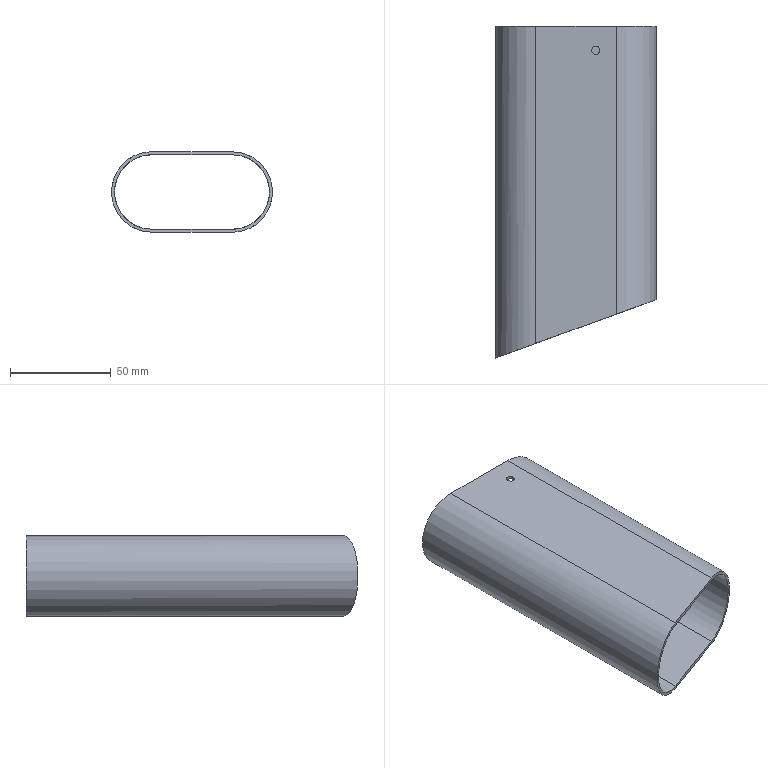Part | STEP file | 6100104L | 1 solid | 11 faces | box 80 x 165 x 40 mm | volume 45327 mm3 | plane 6 | cylinder 5 | commonest cylinder face diameters 37 x2 40 x2 4 x1
STEP:
#1=CARTESIAN_POINT('',(0.,0.,0.));
#2=DIRECTION('',(0.,0.,1.));
#3=DIRECTION('',(1.,0.,0.));
#4=AXIS2_PLACEMENT_3D('',#1,#2,#3);
#5=CARTESIAN_POINT('',(-20.,165.,-20.));
#6=VERTEX_POINT('',#5);
#7=CARTESIAN_POINT('',(-20.,165.,20.));
#8=VERTEX_POINT('',#7);
#9=CARTESIAN_POINT('',(-20.,165.,0.));
#10=DIRECTION('',(0.,1.,0.));
#11=DIRECTION('',(0.,0.,1.));
#12=AXIS2_PLACEMENT_3D('',#9,#10,#11);
#13=CIRCLE('',#12,20.);
#14=CARTESIAN_POINT('',(-20.,165.,0.));
#15=DIRECTION('',(0.,1.,0.));
#16=DIRECTION('',(0.,0.,1.));
#17=AXIS2_PLACEMENT_3D('',#14,#15,#16);
#18=PLANE('',#17);
#19=CARTESIAN_POINT('',(0.,0.));
#20=DIRECTION('',(1.,0.));
#21=AXIS2_PLACEMENT_2D('',#19,#20);
#22=CIRCLE('',#21,20.);
#23=(GEOMETRIC_REPRESENTATION_CONTEXT(2)PARAMETRIC_REPRESENTATION_CONTEXT()REPRESENTATION_CONTEXT('',''));
#24=DEFINITIONAL_REPRESENTATION('',(#22),#23);
#25=PCURVE('',#18,#24);
#26=CARTESIAN_POINT('',(-20.,165.,0.));
#27=DIRECTION('',(0.,-1.,0.));
#28=DIRECTION('',(0.,0.,-1.));
#29=AXIS2_PLACEMENT_3D('',#26,#27,#28);
#30=CYLINDRICAL_SURFACE('',#29,20.);
#31=CARTESIAN_POINT('',(9.425,0.));
#32=DIRECTION('',(-1.,0.));
#33=VECTOR('',#32,1.);
#34=LINE('',#31,#33);
#35=(GEOMETRIC_REPRESENTATION_CONTEXT(2)PARAMETRIC_REPRESENTATION_CONTEXT()REPRESENTATION_CONTEXT('',''));
#36=DEFINITIONAL_REPRESENTATION('',(#34),#35);
#37=PCURVE('',#30,#36);
#38=SURFACE_CURVE('',#13,(#25,#37),.PCURVE_S1.);
#39=EDGE_CURVE('',#6,#8,#38,.T.);
#40=ORIENTED_EDGE('',*,*,#39,.T.);
#41=CARTESIAN_POINT('',(20.,165.,20.));
#42=VERTEX_POINT('',#41);
#43=CARTESIAN_POINT('',(-20.,165.,20.));
#44=DIRECTION('',(1.,0.,0.));
#45=VECTOR('',#44,1.);
#46=LINE('',#43,#45);
#47=CARTESIAN_POINT('',(20.,0.));
#48=DIRECTION('',(0.,1.));
#49=VECTOR('',#48,1.);
#50=LINE('',#47,#49);
#51=(GEOMETRIC_REPRESENTATION_CONTEXT(2)PARAMETRIC_REPRESENTATION_CONTEXT()REPRESENTATION_CONTEXT('',''));
#52=DEFINITIONAL_REPRESENTATION('',(#50),#51);
#53=PCURVE('',#18,#52);
#54=CARTESIAN_POINT('',(-20.,165.,20.));
#55=DIRECTION('',(0.,0.,-1.));
#56=DIRECTION('',(-1.,0.,0.));
#57=AXIS2_PLACEMENT_3D('',#54,#55,#56);
#58=PLANE('',#57);
#59=CARTESIAN_POINT('',(0.,0.));
#60=DIRECTION('',(-1.,0.));
#61=VECTOR('',#60,1.);
#62=LINE('',#59,#61);
#63=(GEOMETRIC_REPRESENTATION_CONTEXT(2)PARAMETRIC_REPRESENTATION_CONTEXT()REPRESENTATION_CONTEXT('',''));
#64=DEFINITIONAL_REPRESENTATION('',(#62),#63);
#65=PCURVE('',#58,#64);
#66=SURFACE_CURVE('',#46,(#53,#65),.PCURVE_S1.);
#67=EDGE_CURVE('',#8,#42,#66,.T.);
#68=ORIENTED_EDGE('',*,*,#67,.T.);
#69=CARTESIAN_POINT('',(20.,165.,-20.));
#70=VERTEX_POINT('',#69);
#71=CARTESIAN_POINT('',(20.,165.,0.));
#72=DIRECTION('',(0.,1.,0.));
#73=DIRECTION('',(0.,0.,1.));
#74=AXIS2_PLACEMENT_3D('',#71,#72,#73);
#75=CIRCLE('',#74,20.);
#76=CARTESIAN_POINT('',(0.,40.));
#77=DIRECTION('',(1.,0.));
#78=AXIS2_PLACEMENT_2D('',#76,#77);
#79=CIRCLE('',#78,20.);
#80=(GEOMETRIC_REPRESENTATION_CONTEXT(2)PARAMETRIC_REPRESENTATION_CONTEXT()REPRESENTATION_CONTEXT('',''));
#81=DEFINITIONAL_REPRESENTATION('',(#79),#80);
#82=PCURVE('',#18,#81);
#83=CARTESIAN_POINT('',(20.,165.,0.));
#84=DIRECTION('',(0.,-1.,0.));
#85=DIRECTION('',(0.,0.,-1.));
#86=AXIS2_PLACEMENT_3D('',#83,#84,#85);
#87=CYLINDRICAL_SURFACE('',#86,20.);
#88=CARTESIAN_POINT('',(3.142,0.));
#89=DIRECTION('',(-1.,0.));
#90=VECTOR('',#89,1.);
#91=LINE('',#88,#90);
#92=(GEOMETRIC_REPRESENTATION_CONTEXT(2)PARAMETRIC_REPRESENTATION_CONTEXT()REPRESENTATION_CONTEXT('',''));
#93=DEFINITIONAL_REPRESENTATION('',(#91),#92);
#94=PCURVE('',#87,#93);
#95=SURFACE_CURVE('',#75,(#82,#94),.PCURVE_S1.);
#96=EDGE_CURVE('',#42,#70,#95,.T.);
#97=ORIENTED_EDGE('',*,*,#96,.T.);
#98=CARTESIAN_POINT('',(-20.,165.,-20.));
#99=DIRECTION('',(-1.,0.,0.));
#100=VECTOR('',#99,1.);
#101=LINE('',#98,#100);
#102=CARTESIAN_POINT('',(-20.,0.));
#103=DIRECTION('',(0.,-1.));
#104=VECTOR('',#103,1.);
#105=LINE('',#102,#104);
#106=(GEOMETRIC_REPRESENTATION_CONTEXT(2)PARAMETRIC_REPRESENTATION_CONTEXT()REPRESENTATION_CONTEXT('',''));
#107=DEFINITIONAL_REPRESENTATION('',(#105),#106);
#108=PCURVE('',#18,#107);
#109=CARTESIAN_POINT('',(-20.,165.,-20.));
#110=DIRECTION('',(0.,0.,1.));
#111=DIRECTION('',(1.,0.,0.));
#112=AXIS2_PLACEMENT_3D('',#109,#110,#111);
#113=PLANE('',#112);
#114=CARTESIAN_POINT('',(0.,0.));
#115=DIRECTION('',(-1.,0.));
#116=VECTOR('',#115,1.);
#117=LINE('',#114,#116);
#118=(GEOMETRIC_REPRESENTATION_CONTEXT(2)PARAMETRIC_REPRESENTATION_CONTEXT()REPRESENTATION_CONTEXT('',''));
#119=DEFINITIONAL_REPRESENTATION('',(#117),#118);
#120=PCURVE('',#113,#119);
#121=SURFACE_CURVE('',#101,(#108,#120),.PCURVE_S1.);
#122=EDGE_CURVE('',#70,#6,#121,.T.);
#123=ORIENTED_EDGE('',*,*,#122,.T.);
#124=EDGE_LOOP('',(#40,#68,#97,#123));
#125=FACE_BOUND('',#124,.T.);
#126=CARTESIAN_POINT('',(-20.,165.,18.5));
#127=VERTEX_POINT('',#126);
#128=CARTESIAN_POINT('',(20.,165.,18.5));
#129=VERTEX_POINT('',#128);
#130=CARTESIAN_POINT('',(-20.,165.,18.5));
#131=DIRECTION('',(1.,0.,0.));
#132=VECTOR('',#131,1.);
#133=LINE('',#130,#132);
#134=CARTESIAN_POINT('',(18.5,0.));
#135=DIRECTION('',(0.,1.));
#136=VECTOR('',#135,1.);
#137=LINE('',#134,#136);
#138=(GEOMETRIC_REPRESENTATION_CONTEXT(2)PARAMETRIC_REPRESENTATION_CONTEXT()REPRESENTATION_CONTEXT('',''));
#139=DEFINITIONAL_REPRESENTATION('',(#137),#138);
#140=PCURVE('',#18,#139);
#141=CARTESIAN_POINT('',(-20.,165.,18.5));
#142=DIRECTION('',(0.,0.,-1.));
#143=DIRECTION('',(-1.,0.,0.));
#144=AXIS2_PLACEMENT_3D('',#141,#142,#143);
#145=PLANE('',#144);
#146=CARTESIAN_POINT('',(0.,0.));
#147=DIRECTION('',(-1.,0.));
#148=VECTOR('',#147,1.);
#149=LINE('',#146,#148);
#150=(GEOMETRIC_REPRESENTATION_CONTEXT(2)PARAMETRIC_REPRESENTATION_CONTEXT()REPRESENTATION_CONTEXT('',''));
#151=DEFINITIONAL_REPRESENTATION('',(#149),#150);
#152=PCURVE('',#145,#151);
#153=SURFACE_CURVE('',#133,(#140,#152),.PCURVE_S1.);
#154=EDGE_CURVE('',#127,#129,#153,.T.);
#155=ORIENTED_EDGE('',*,*,#154,.F.);
#156=CARTESIAN_POINT('',(-20.,165.,-18.5));
#157=VERTEX_POINT('',#156);
#158=CARTESIAN_POINT('',(-20.,165.,0.));
#159=DIRECTION('',(0.,1.,0.));
#160=DIRECTION('',(0.,0.,1.));
#161=AXIS2_PLACEMENT_3D('',#158,#159,#160);
#162=CIRCLE('',#161,18.5);
#163=CARTESIAN_POINT('',(0.,0.));
#164=DIRECTION('',(1.,0.));
#165=AXIS2_PLACEMENT_2D('',#163,#164);
#166=CIRCLE('',#165,18.5);
#167=(GEOMETRIC_REPRESENTATION_CONTEXT(2)PARAMETRIC_REPRESENTATION_CONTEXT()REPRESENTATION_CONTEXT('',''));
#168=DEFINITIONAL_REPRESENTATION('',(#166),#167);
#169=PCURVE('',#18,#168);
#170=CARTESIAN_POINT('',(-20.,165.,0.));
#171=DIRECTION('',(0.,-1.,0.));
#172=DIRECTION('',(0.,0.,-1.));
#173=AXIS2_PLACEMENT_3D('',#170,#171,#172);
#174=CYLINDRICAL_SURFACE('',#173,18.5);
#175=CARTESIAN_POINT('',(9.425,0.));
#176=DIRECTION('',(-1.,0.));
#177=VECTOR('',#176,1.);
#178=LINE('',#175,#177);
#179=(GEOMETRIC_REPRESENTATION_CONTEXT(2)PARAMETRIC_REPRESENTATION_CONTEXT()REPRESENTATION_CONTEXT('',''));
#180=DEFINITIONAL_REPRESENTATION('',(#178),#179);
#181=PCURVE('',#174,#180);
#182=SURFACE_CURVE('',#162,(#169,#181),.PCURVE_S1.);
#183=EDGE_CURVE('',#157,#127,#182,.T.);
#184=ORIENTED_EDGE('',*,*,#183,.F.);
#185=CARTESIAN_POINT('',(20.,165.,-18.5));
#186=VERTEX_POINT('',#185);
#187=CARTESIAN_POINT('',(-20.,165.,-18.5));
#188=DIRECTION('',(-1.,0.,0.));
#189=VECTOR('',#188,1.);
#190=LINE('',#187,#189);
#191=CARTESIAN_POINT('',(-18.5,0.));
#192=DIRECTION('',(0.,-1.));
#193=VECTOR('',#192,1.);
#194=LINE('',#191,#193);
#195=(GEOMETRIC_REPRESENTATION_CONTEXT(2)PARAMETRIC_REPRESENTATION_CONTEXT()REPRESENTATION_CONTEXT('',''));
#196=DEFINITIONAL_REPRESENTATION('',(#194),#195);
#197=PCURVE('',#18,#196);
#198=CARTESIAN_POINT('',(-20.,165.,-18.5));
#199=DIRECTION('',(0.,0.,1.));
#200=DIRECTION('',(1.,0.,0.));
#201=AXIS2_PLACEMENT_3D('',#198,#199,#200);
#202=PLANE('',#201);
#203=CARTESIAN_POINT('',(0.,0.));
#204=DIRECTION('',(-1.,0.));
#205=VECTOR('',#204,1.);
#206=LINE('',#203,#205);
#207=(GEOMETRIC_REPRESENTATION_CONTEXT(2)PARAMETRIC_REPRESENTATION_CONTEXT()REPRESENTATION_CONTEXT('',''));
#208=DEFINITIONAL_REPRESENTATION('',(#206),#207);
#209=PCURVE('',#202,#208);
#210=SURFACE_CURVE('',#190,(#197,#209),.PCURVE_S1.);
#211=EDGE_CURVE('',#186,#157,#210,.T.);
#212=ORIENTED_EDGE('',*,*,#211,.F.);
#213=CARTESIAN_POINT('',(20.,165.,0.));
#214=DIRECTION('',(0.,1.,0.));
#215=DIRECTION('',(0.,0.,1.));
#216=AXIS2_PLACEMENT_3D('',#213,#214,#215);
#217=CIRCLE('',#216,18.5);
#218=CARTESIAN_POINT('',(0.,40.));
#219=DIRECTION('',(1.,0.));
#220=AXIS2_PLACEMENT_2D('',#218,#219);
#221=CIRCLE('',#220,18.5);
#222=(GEOMETRIC_REPRESENTATION_CONTEXT(2)PARAMETRIC_REPRESENTATION_CONTEXT()REPRESENTATION_CONTEXT('',''));
#223=DEFINITIONAL_REPRESENTATION('',(#221),#222);
#224=PCURVE('',#18,#223);
#225=CARTESIAN_POINT('',(20.,165.,0.));
#226=DIRECTION('',(0.,-1.,0.));
#227=DIRECTION('',(0.,0.,-1.));
#228=AXIS2_PLACEMENT_3D('',#225,#226,#227);
#229=CYLINDRICAL_SURFACE('',#228,18.5);
#230=CARTESIAN_POINT('',(3.142,0.));
#231=DIRECTION('',(-1.,0.));
#232=VECTOR('',#231,1.);
#233=LINE('',#230,#232);
#234=(GEOMETRIC_REPRESENTATION_CONTEXT(2)PARAMETRIC_REPRESENTATION_CONTEXT()REPRESENTATION_CONTEXT('',''));
#235=DEFINITIONAL_REPRESENTATION('',(#233),#234);
#236=PCURVE('',#229,#235);
#237=SURFACE_CURVE('',#217,(#224,#236),.PCURVE_S1.);
#238=EDGE_CURVE('',#129,#186,#237,.T.);
#239=ORIENTED_EDGE('',*,*,#238,.F.);
#240=EDGE_LOOP('',(#155,#184,#212,#239));
#241=FACE_BOUND('',#240,.T.);
#242=ADVANCED_FACE('',(#125,#241),#18,.T.);
#243=CARTESIAN_POINT('',(-20.,7.279,-20.));
#244=VERTEX_POINT('',#243);
#245=CARTESIAN_POINT('',(-20.,165.,-20.));
#246=DIRECTION('',(0.,-1.,0.));
#247=VECTOR('',#246,1.);
#248=LINE('',#245,#247);
#249=CARTESIAN_POINT('',(6.283,0.));
#250=DIRECTION('',(0.,1.));
#251=VECTOR('',#250,1.);
#252=LINE('',#249,#251);
#253=(GEOMETRIC_REPRESENTATION_CONTEXT(2)PARAMETRIC_REPRESENTATION_CONTEXT()REPRESENTATION_CONTEXT('',''));
#254=DEFINITIONAL_REPRESENTATION('',(#252),#253);
#255=PCURVE('',#30,#254);
#256=CARTESIAN_POINT('',(0.,0.));
#257=DIRECTION('',(0.,-1.));
#258=VECTOR('',#257,1.);
#259=LINE('',#256,#258);
#260=(GEOMETRIC_REPRESENTATION_CONTEXT(2)PARAMETRIC_REPRESENTATION_CONTEXT()REPRESENTATION_CONTEXT('',''));
#261=DEFINITIONAL_REPRESENTATION('',(#259),#260);
#262=PCURVE('',#113,#261);
#263=SURFACE_CURVE('',#248,(#255,#262),.PCURVE_S1.);
#264=EDGE_CURVE('',#6,#244,#263,.T.);
#265=ORIENTED_EDGE('',*,*,#264,.T.);
#266=CARTESIAN_POINT('',(-20.,7.279,20.));
#267=VERTEX_POINT('',#266);
#268=CARTESIAN_POINT('',(-20.,7.279,-20.));
#269=CARTESIAN_POINT('',(-60.,-7.279,-20.));
#270=CARTESIAN_POINT('',(-60.,-7.279,20.));
#271=CARTESIAN_POINT('',(-20.,7.279,20.));
#272=(BOUNDED_CURVE()B_SPLINE_CURVE(3,(#268,#269,#270,#271),.UNSPECIFIED.,.F.,.F.)B_SPLINE_CURVE_WITH_KNOTS((4,4),(4.712,7.854),.PIECEWISE_BEZIER_KNOTS.)CURVE()GEOMETRIC_REPRESENTATION_ITEM()RATIONAL_B_SPLINE_CURVE((1.,0.3333,0.3333,1.))REPRESENTATION_ITEM(''));
#273=CARTESIAN_POINT('',(6.283,157.721));
#274=CARTESIAN_POINT('',(6.253,157.941));
#275=CARTESIAN_POINT('',(6.19,158.403));
#276=CARTESIAN_POINT('',(6.085,159.153));
#277=CARTESIAN_POINT('',(5.972,159.957));
#278=CARTESIAN_POINT('',(5.848,160.8));
#279=CARTESIAN_POINT('',(5.713,161.664));
#280=CARTESIAN_POINT('',(5.567,162.516));
#281=CARTESIAN_POINT('',(5.412,163.316));
#282=CARTESIAN_POINT('',(5.246,164.017));
#283=CARTESIAN_POINT('',(5.073,164.567));
#284=CARTESIAN_POINT('',(4.894,164.919));
#285=CARTESIAN_POINT('',(4.712,165.04));
#286=CARTESIAN_POINT('',(4.531,164.919));
#287=CARTESIAN_POINT('',(4.352,164.567));
#288=CARTESIAN_POINT('',(4.179,164.017));
#289=CARTESIAN_POINT('',(4.013,163.316));
#290=CARTESIAN_POINT('',(3.857,162.516));
#291=CARTESIAN_POINT('',(3.712,161.664));
#292=CARTESIAN_POINT('',(3.577,160.8));
#293=CARTESIAN_POINT('',(3.453,159.957));
#294=CARTESIAN_POINT('',(3.339,159.153));
#295=CARTESIAN_POINT('',(3.235,158.403));
#296=CARTESIAN_POINT('',(3.172,157.941));
#297=CARTESIAN_POINT('',(3.142,157.721));
#298=B_SPLINE_CURVE_WITH_KNOTS('',3,(#273,#274,#275,#276,#277,#278,#279,#280,#281,#282,#283,#284,#285,#286,#287,#288,#289,#290,#291,#292,#293,#294,#295,#296,#297),.UNSPECIFIED.,.F.,.F.,(4,1,1,1,1,1,1,1,1,1,1,1,1,1,1,1,1,1,1,1,1,1,4),(4.712,4.855,4.998,5.141,5.284,5.426,5.569,5.712,5.855,5.998,6.14,6.283,6.426,6.569,6.712,6.854,6.997,7.14,7.283,7.426,7.568,7.711,7.854),.QUASI_UNIFORM_KNOTS.);
#299=(GEOMETRIC_REPRESENTATION_CONTEXT(2)PARAMETRIC_REPRESENTATION_CONTEXT()REPRESENTATION_CONTEXT('',''));
#300=DEFINITIONAL_REPRESENTATION('',(#298),#299);
#301=PCURVE('',#30,#300);
#302=CARTESIAN_POINT('',(-40.,0.,-40.));
#303=DIRECTION('',(-0.342,0.9397,0.));
#304=DIRECTION('',(-0.9397,-0.342,0.));
#305=AXIS2_PLACEMENT_3D('',#302,#303,#304);
#306=PLANE('',#305);
#307=CARTESIAN_POINT('',(-21.284,20.));
#308=CARTESIAN_POINT('',(21.284,20.));
#309=CARTESIAN_POINT('',(21.284,60.));
#310=CARTESIAN_POINT('',(-21.284,60.));
#311=(BOUNDED_CURVE()B_SPLINE_CURVE(3,(#307,#308,#309,#310),.UNSPECIFIED.,.F.,.F.)B_SPLINE_CURVE_WITH_KNOTS((4,4),(4.712,7.854),.PIECEWISE_BEZIER_KNOTS.)CURVE()GEOMETRIC_REPRESENTATION_ITEM()RATIONAL_B_SPLINE_CURVE((1.,0.3333,0.3333,1.))REPRESENTATION_ITEM(''));
#312=(GEOMETRIC_REPRESENTATION_CONTEXT(2)PARAMETRIC_REPRESENTATION_CONTEXT()REPRESENTATION_CONTEXT('',''));
#313=DEFINITIONAL_REPRESENTATION('',(#311),#312);
#314=PCURVE('',#306,#313);
#315=SURFACE_CURVE('',#272,(#301,#314),.PCURVE_S1.);
#316=EDGE_CURVE('',#244,#267,#315,.T.);
#317=ORIENTED_EDGE('',*,*,#316,.T.);
#318=CARTESIAN_POINT('',(-20.,165.,20.));
#319=DIRECTION('',(0.,-1.,0.));
#320=VECTOR('',#319,1.);
#321=LINE('',#318,#320);
#322=CARTESIAN_POINT('',(3.142,0.));
#323=DIRECTION('',(0.,1.));
#324=VECTOR('',#323,1.);
#325=LINE('',#322,#324);
#326=(GEOMETRIC_REPRESENTATION_CONTEXT(2)PARAMETRIC_REPRESENTATION_CONTEXT()REPRESENTATION_CONTEXT('',''));
#327=DEFINITIONAL_REPRESENTATION('',(#325),#326);
#328=PCURVE('',#30,#327);
#329=CARTESIAN_POINT('',(0.,0.));
#330=DIRECTION('',(0.,-1.));
#331=VECTOR('',#330,1.);
#332=LINE('',#329,#331);
#333=(GEOMETRIC_REPRESENTATION_CONTEXT(2)PARAMETRIC_REPRESENTATION_CONTEXT()REPRESENTATION_CONTEXT('',''));
#334=DEFINITIONAL_REPRESENTATION('',(#332),#333);
#335=PCURVE('',#58,#334);
#336=SURFACE_CURVE('',#321,(#328,#335),.PCURVE_S1.);
#337=EDGE_CURVE('',#8,#267,#336,.T.);
#338=ORIENTED_EDGE('',*,*,#337,.F.);
#339=ORIENTED_EDGE('',*,*,#39,.F.);
#340=EDGE_LOOP('',(#265,#317,#338,#339));
#341=FACE_BOUND('',#340,.T.);
#342=ADVANCED_FACE('',(#341),#30,.T.);
#343=CARTESIAN_POINT('',(11.87,152.93,20.));
#344=VERTEX_POINT('',#343);
#345=CARTESIAN_POINT('',(9.87,152.93,20.));
#346=DIRECTION('',(0.,0.,1.));
#347=DIRECTION('',(1.,0.,0.));
#348=AXIS2_PLACEMENT_3D('',#345,#346,#347);
#349=CIRCLE('',#348,2.);
#350=CARTESIAN_POINT('',(-31.87,-12.07));
#351=CARTESIAN_POINT('',(-31.87,-8.606));
#352=CARTESIAN_POINT('',(-28.87,-10.338));
#353=CARTESIAN_POINT('',(-25.87,-12.07));
#354=CARTESIAN_POINT('',(-28.87,-13.802));
#355=CARTESIAN_POINT('',(-31.87,-15.534));
#356=CARTESIAN_POINT('',(-31.87,-12.07));
#357=(BOUNDED_CURVE()B_SPLINE_CURVE(2,(#350,#351,#352,#353,#354,#355,#356),.UNSPECIFIED.,.T.,.F.)B_SPLINE_CURVE_WITH_KNOTS((1,2,2,2,2,1),(-2.094,0.,2.094,4.189,6.283,8.378),.UNSPECIFIED.)CURVE()GEOMETRIC_REPRESENTATION_ITEM()RATIONAL_B_SPLINE_CURVE((1.,0.5,1.,0.5,1.,0.5,1.))REPRESENTATION_ITEM(''));
#358=(GEOMETRIC_REPRESENTATION_CONTEXT(2)PARAMETRIC_REPRESENTATION_CONTEXT()REPRESENTATION_CONTEXT('',''));
#359=DEFINITIONAL_REPRESENTATION('',(#357),#358);
#360=PCURVE('',#58,#359);
#361=CARTESIAN_POINT('',(9.87,152.93,10.));
#362=DIRECTION('',(0.,0.,1.));
#363=DIRECTION('',(1.,0.,0.));
#364=AXIS2_PLACEMENT_3D('',#361,#362,#363);
#365=CYLINDRICAL_SURFACE('',#364,2.);
#366=CARTESIAN_POINT('',(0.,10.));
#367=DIRECTION('',(1.,0.));
#368=VECTOR('',#367,1.);
#369=LINE('',#366,#368);
#370=(GEOMETRIC_REPRESENTATION_CONTEXT(2)PARAMETRIC_REPRESENTATION_CONTEXT()REPRESENTATION_CONTEXT('',''));
#371=DEFINITIONAL_REPRESENTATION('',(#369),#370);
#372=PCURVE('',#365,#371);
#373=SURFACE_CURVE('',#349,(#360,#372),.PCURVE_S1.);
#374=EDGE_CURVE('',#344,#344,#373,.T.);
#375=ORIENTED_EDGE('',*,*,#374,.F.);
#376=EDGE_LOOP('',(#375));
#377=FACE_BOUND('',#376,.T.);
#378=ORIENTED_EDGE('',*,*,#337,.T.);
#379=CARTESIAN_POINT('',(20.,21.838,20.));
#380=VERTEX_POINT('',#379);
#381=CARTESIAN_POINT('',(30.69,25.729,20.));
#382=DIRECTION('',(0.9397,0.342,0.));
#383=VECTOR('',#382,1.);
#384=LINE('',#381,#383);
#385=CARTESIAN_POINT('',(-50.69,-139.271));
#386=DIRECTION('',(-0.9397,0.342));
#387=VECTOR('',#386,1.);
#388=LINE('',#385,#387);
#389=(GEOMETRIC_REPRESENTATION_CONTEXT(2)PARAMETRIC_REPRESENTATION_CONTEXT()REPRESENTATION_CONTEXT('',''));
#390=DEFINITIONAL_REPRESENTATION('',(#388),#389);
#391=PCURVE('',#58,#390);
#392=CARTESIAN_POINT('',(-75.227,60.));
#393=DIRECTION('',(-1.,0.));
#394=VECTOR('',#393,1.);
#395=LINE('',#392,#394);
#396=(GEOMETRIC_REPRESENTATION_CONTEXT(2)PARAMETRIC_REPRESENTATION_CONTEXT()REPRESENTATION_CONTEXT('',''));
#397=DEFINITIONAL_REPRESENTATION('',(#395),#396);
#398=PCURVE('',#306,#397);
#399=SURFACE_CURVE('',#384,(#391,#398),.PCURVE_S1.);
#400=EDGE_CURVE('',#267,#380,#399,.T.);
#401=ORIENTED_EDGE('',*,*,#400,.T.);
#402=CARTESIAN_POINT('',(20.,165.,20.));
#403=DIRECTION('',(0.,-1.,0.));
#404=VECTOR('',#403,1.);
#405=LINE('',#402,#404);
#406=CARTESIAN_POINT('',(-40.,0.));
#407=DIRECTION('',(0.,-1.));
#408=VECTOR('',#407,1.);
#409=LINE('',#406,#408);
#410=(GEOMETRIC_REPRESENTATION_CONTEXT(2)PARAMETRIC_REPRESENTATION_CONTEXT()REPRESENTATION_CONTEXT('',''));
#411=DEFINITIONAL_REPRESENTATION('',(#409),#410);
#412=PCURVE('',#58,#411);
#413=CARTESIAN_POINT('',(3.142,0.));
#414=DIRECTION('',(0.,1.));
#415=VECTOR('',#414,1.);
#416=LINE('',#413,#415);
#417=(GEOMETRIC_REPRESENTATION_CONTEXT(2)PARAMETRIC_REPRESENTATION_CONTEXT()REPRESENTATION_CONTEXT('',''));
#418=DEFINITIONAL_REPRESENTATION('',(#416),#417);
#419=PCURVE('',#87,#418);
#420=SURFACE_CURVE('',#405,(#412,#419),.PCURVE_S1.);
#421=EDGE_CURVE('',#42,#380,#420,.T.);
#422=ORIENTED_EDGE('',*,*,#421,.F.);
#423=ORIENTED_EDGE('',*,*,#67,.F.);
#424=EDGE_LOOP('',(#378,#401,#422,#423));
#425=FACE_BOUND('',#424,.T.);
#426=ADVANCED_FACE('',(#377,#425),#58,.F.);
#427=CARTESIAN_POINT('',(20.,21.838,-20.));
#428=VERTEX_POINT('',#427);
#429=CARTESIAN_POINT('',(20.,21.838,20.));
#430=CARTESIAN_POINT('',(60.,36.397,20.));
#431=CARTESIAN_POINT('',(60.,36.397,-20.));
#432=CARTESIAN_POINT('',(20.,21.838,-20.));
#433=(BOUNDED_CURVE()B_SPLINE_CURVE(3,(#429,#430,#431,#432),.UNSPECIFIED.,.F.,.F.)B_SPLINE_CURVE_WITH_KNOTS((4,4),(1.571,4.712),.PIECEWISE_BEZIER_KNOTS.)CURVE()GEOMETRIC_REPRESENTATION_ITEM()RATIONAL_B_SPLINE_CURVE((1.,0.3333,0.3333,1.))REPRESENTATION_ITEM(''));
#434=CARTESIAN_POINT('',(3.142,143.162));
#435=CARTESIAN_POINT('',(3.111,142.942));
#436=CARTESIAN_POINT('',(3.048,142.48));
#437=CARTESIAN_POINT('',(2.944,141.729));
#438=CARTESIAN_POINT('',(2.83,140.926));
#439=CARTESIAN_POINT('',(2.706,140.082));
#440=CARTESIAN_POINT('',(2.571,139.219));
#441=CARTESIAN_POINT('',(2.426,138.367));
#442=CARTESIAN_POINT('',(2.27,137.566));
#443=CARTESIAN_POINT('',(2.105,136.865));
#444=CARTESIAN_POINT('',(1.931,136.315));
#445=CARTESIAN_POINT('',(1.753,135.963));
#446=CARTESIAN_POINT('',(1.571,135.842));
#447=CARTESIAN_POINT('',(1.389,135.963));
#448=CARTESIAN_POINT('',(1.21,136.315));
#449=CARTESIAN_POINT('',(1.037,136.865));
#450=CARTESIAN_POINT('',(0.8717,137.566));
#451=CARTESIAN_POINT('',(0.7158,138.367));
#452=CARTESIAN_POINT('',(0.5703,139.219));
#453=CARTESIAN_POINT('',(0.4356,140.082));
#454=CARTESIAN_POINT('',(0.3115,140.926));
#455=CARTESIAN_POINT('',(0.1977,141.729));
#456=CARTESIAN_POINT('',(0.09367,142.48));
#457=CARTESIAN_POINT('',(0.0303,142.942));
#458=CARTESIAN_POINT('',(0.,143.162));
#459=B_SPLINE_CURVE_WITH_KNOTS('',3,(#434,#435,#436,#437,#438,#439,#440,#441,#442,#443,#444,#445,#446,#447,#448,#449,#450,#451,#452,#453,#454,#455,#456,#457,#458),.UNSPECIFIED.,.F.,.F.,(4,1,1,1,1,1,1,1,1,1,1,1,1,1,1,1,1,1,1,1,1,1,4),(1.571,1.714,1.856,1.999,2.142,2.285,2.428,2.57,2.713,2.856,2.999,3.142,3.284,3.427,3.57,3.713,3.856,3.998,4.141,4.284,4.427,4.57,4.712),.QUASI_UNIFORM_KNOTS.);
#460=(GEOMETRIC_REPRESENTATION_CONTEXT(2)PARAMETRIC_REPRESENTATION_CONTEXT()REPRESENTATION_CONTEXT('',''));
#461=DEFINITIONAL_REPRESENTATION('',(#459),#460);
#462=PCURVE('',#87,#461);
#463=CARTESIAN_POINT('',(-63.851,60.));
#464=CARTESIAN_POINT('',(-106.418,60.));
#465=CARTESIAN_POINT('',(-106.418,20.));
#466=CARTESIAN_POINT('',(-63.851,20.));
#467=(BOUNDED_CURVE()B_SPLINE_CURVE(3,(#463,#464,#465,#466),.UNSPECIFIED.,.F.,.F.)B_SPLINE_CURVE_WITH_KNOTS((4,4),(1.571,4.712),.PIECEWISE_BEZIER_KNOTS.)CURVE()GEOMETRIC_REPRESENTATION_ITEM()RATIONAL_B_SPLINE_CURVE((1.,0.3333,0.3333,1.))REPRESENTATION_ITEM(''));
#468=(GEOMETRIC_REPRESENTATION_CONTEXT(2)PARAMETRIC_REPRESENTATION_CONTEXT()REPRESENTATION_CONTEXT('',''));
#469=DEFINITIONAL_REPRESENTATION('',(#467),#468);
#470=PCURVE('',#306,#469);
#471=SURFACE_CURVE('',#433,(#462,#470),.PCURVE_S1.);
#472=EDGE_CURVE('',#380,#428,#471,.T.);
#473=ORIENTED_EDGE('',*,*,#472,.T.);
#474=CARTESIAN_POINT('',(20.,165.,-20.));
#475=DIRECTION('',(0.,-1.,0.));
#476=VECTOR('',#475,1.);
#477=LINE('',#474,#476);
#478=CARTESIAN_POINT('',(0.,0.));
#479=DIRECTION('',(0.,1.));
#480=VECTOR('',#479,1.);
#481=LINE('',#478,#480);
#482=(GEOMETRIC_REPRESENTATION_CONTEXT(2)PARAMETRIC_REPRESENTATION_CONTEXT()REPRESENTATION_CONTEXT('',''));
#483=DEFINITIONAL_REPRESENTATION('',(#481),#482);
#484=PCURVE('',#87,#483);
#485=CARTESIAN_POINT('',(40.,0.));
#486=DIRECTION('',(0.,-1.));
#487=VECTOR('',#486,1.);
#488=LINE('',#485,#487);
#489=(GEOMETRIC_REPRESENTATION_CONTEXT(2)PARAMETRIC_REPRESENTATION_CONTEXT()REPRESENTATION_CONTEXT('',''));
#490=DEFINITIONAL_REPRESENTATION('',(#488),#489);
#491=PCURVE('',#113,#490);
#492=SURFACE_CURVE('',#477,(#484,#491),.PCURVE_S1.);
#493=EDGE_CURVE('',#70,#428,#492,.T.);
#494=ORIENTED_EDGE('',*,*,#493,.F.);
#495=ORIENTED_EDGE('',*,*,#96,.F.);
#496=ORIENTED_EDGE('',*,*,#421,.T.);
#497=EDGE_LOOP('',(#473,#494,#495,#496));
#498=FACE_BOUND('',#497,.T.);
#499=ADVANCED_FACE('',(#498),#87,.T.);
#500=ORIENTED_EDGE('',*,*,#493,.T.);
#501=CARTESIAN_POINT('',(30.69,25.729,-20.));
#502=DIRECTION('',(-0.9397,-0.342,0.));
#503=VECTOR('',#502,1.);
#504=LINE('',#501,#503);
#505=CARTESIAN_POINT('',(50.69,-139.271));
#506=DIRECTION('',(-0.9397,-0.342));
#507=VECTOR('',#506,1.);
#508=LINE('',#505,#507);
#509=(GEOMETRIC_REPRESENTATION_CONTEXT(2)PARAMETRIC_REPRESENTATION_CONTEXT()REPRESENTATION_CONTEXT('',''));
#510=DEFINITIONAL_REPRESENTATION('',(#508),#509);
#511=PCURVE('',#113,#510);
#512=CARTESIAN_POINT('',(-75.227,20.));
#513=DIRECTION('',(1.,0.));
#514=VECTOR('',#513,1.);
#515=LINE('',#512,#514);
#516=(GEOMETRIC_REPRESENTATION_CONTEXT(2)PARAMETRIC_REPRESENTATION_CONTEXT()REPRESENTATION_CONTEXT('',''));
#517=DEFINITIONAL_REPRESENTATION('',(#515),#516);
#518=PCURVE('',#306,#517);
#519=SURFACE_CURVE('',#504,(#511,#518),.PCURVE_S1.);
#520=EDGE_CURVE('',#428,#244,#519,.T.);
#521=ORIENTED_EDGE('',*,*,#520,.T.);
#522=ORIENTED_EDGE('',*,*,#264,.F.);
#523=ORIENTED_EDGE('',*,*,#122,.F.);
#524=EDGE_LOOP('',(#500,#521,#522,#523));
#525=FACE_BOUND('',#524,.T.);
#526=ADVANCED_FACE('',(#525),#113,.F.);
#527=CARTESIAN_POINT('',(-20.,7.279,18.5));
#528=VERTEX_POINT('',#527);
#529=CARTESIAN_POINT('',(-20.,165.,18.5));
#530=DIRECTION('',(0.,-1.,0.));
#531=VECTOR('',#530,1.);
#532=LINE('',#529,#531);
#533=CARTESIAN_POINT('',(3.142,0.));
#534=DIRECTION('',(0.,1.));
#535=VECTOR('',#534,1.);
#536=LINE('',#533,#535);
#537=(GEOMETRIC_REPRESENTATION_CONTEXT(2)PARAMETRIC_REPRESENTATION_CONTEXT()REPRESENTATION_CONTEXT('',''));
#538=DEFINITIONAL_REPRESENTATION('',(#536),#537);
#539=PCURVE('',#174,#538);
#540=CARTESIAN_POINT('',(0.,0.));
#541=DIRECTION('',(0.,-1.));
#542=VECTOR('',#541,1.);
#543=LINE('',#540,#542);
#544=(GEOMETRIC_REPRESENTATION_CONTEXT(2)PARAMETRIC_REPRESENTATION_CONTEXT()REPRESENTATION_CONTEXT('',''));
#545=DEFINITIONAL_REPRESENTATION('',(#543),#544);
#546=PCURVE('',#145,#545);
#547=SURFACE_CURVE('',#532,(#539,#546),.PCURVE_S1.);
#548=EDGE_CURVE('',#127,#528,#547,.T.);
#549=ORIENTED_EDGE('',*,*,#548,.F.);
#550=ORIENTED_EDGE('',*,*,#183,.F.);
#551=CARTESIAN_POINT('',(-20.,7.279,-18.5));
#552=VERTEX_POINT('',#551);
#553=CARTESIAN_POINT('',(-20.,165.,-18.5));
#554=DIRECTION('',(0.,-1.,0.));
#555=VECTOR('',#554,1.);
#556=LINE('',#553,#555);
#557=CARTESIAN_POINT('',(6.283,0.));
#558=DIRECTION('',(0.,1.));
#559=VECTOR('',#558,1.);
#560=LINE('',#557,#559);
#561=(GEOMETRIC_REPRESENTATION_CONTEXT(2)PARAMETRIC_REPRESENTATION_CONTEXT()REPRESENTATION_CONTEXT('',''));
#562=DEFINITIONAL_REPRESENTATION('',(#560),#561);
#563=PCURVE('',#174,#562);
#564=CARTESIAN_POINT('',(0.,0.));
#565=DIRECTION('',(0.,-1.));
#566=VECTOR('',#565,1.);
#567=LINE('',#564,#566);
#568=(GEOMETRIC_REPRESENTATION_CONTEXT(2)PARAMETRIC_REPRESENTATION_CONTEXT()REPRESENTATION_CONTEXT('',''));
#569=DEFINITIONAL_REPRESENTATION('',(#567),#568);
#570=PCURVE('',#202,#569);
#571=SURFACE_CURVE('',#556,(#563,#570),.PCURVE_S1.);
#572=EDGE_CURVE('',#157,#552,#571,.T.);
#573=ORIENTED_EDGE('',*,*,#572,.T.);
#574=CARTESIAN_POINT('',(-20.,7.279,-18.5));
#575=CARTESIAN_POINT('',(-57.,-6.187,-18.5));
#576=CARTESIAN_POINT('',(-57.,-6.187,18.5));
#577=CARTESIAN_POINT('',(-20.,7.279,18.5));
#578=(BOUNDED_CURVE()B_SPLINE_CURVE(3,(#574,#575,#576,#577),.UNSPECIFIED.,.F.,.F.)B_SPLINE_CURVE_WITH_KNOTS((4,4),(4.712,7.854),.PIECEWISE_BEZIER_KNOTS.)CURVE()GEOMETRIC_REPRESENTATION_ITEM()RATIONAL_B_SPLINE_CURVE((1.,0.3333,0.3333,1.))REPRESENTATION_ITEM(''));
#579=CARTESIAN_POINT('',(6.283,157.721));
#580=CARTESIAN_POINT('',(6.253,157.924));
#581=CARTESIAN_POINT('',(6.19,158.352));
#582=CARTESIAN_POINT('',(6.085,159.046));
#583=CARTESIAN_POINT('',(5.972,159.789));
#584=CARTESIAN_POINT('',(5.848,160.569));
#585=CARTESIAN_POINT('',(5.713,161.368));
#586=CARTESIAN_POINT('',(5.567,162.156));
#587=CARTESIAN_POINT('',(5.412,162.897));
#588=CARTESIAN_POINT('',(5.246,163.545));
#589=CARTESIAN_POINT('',(5.073,164.054));
#590=CARTESIAN_POINT('',(4.894,164.379));
#591=CARTESIAN_POINT('',(4.712,164.491));
#592=CARTESIAN_POINT('',(4.531,164.379));
#593=CARTESIAN_POINT('',(4.352,164.054));
#594=CARTESIAN_POINT('',(4.179,163.545));
#595=CARTESIAN_POINT('',(4.013,162.897));
#596=CARTESIAN_POINT('',(3.857,162.156));
#597=CARTESIAN_POINT('',(3.712,161.368));
#598=CARTESIAN_POINT('',(3.577,160.569));
#599=CARTESIAN_POINT('',(3.453,159.789));
#600=CARTESIAN_POINT('',(3.339,159.046));
#601=CARTESIAN_POINT('',(3.235,158.352));
#602=CARTESIAN_POINT('',(3.172,157.924));
#603=CARTESIAN_POINT('',(3.142,157.721));
#604=B_SPLINE_CURVE_WITH_KNOTS('',3,(#579,#580,#581,#582,#583,#584,#585,#586,#587,#588,#589,#590,#591,#592,#593,#594,#595,#596,#597,#598,#599,#600,#601,#602,#603),.UNSPECIFIED.,.F.,.F.,(4,1,1,1,1,1,1,1,1,1,1,1,1,1,1,1,1,1,1,1,1,1,4),(4.712,4.855,4.998,5.141,5.284,5.426,5.569,5.712,5.855,5.998,6.14,6.283,6.426,6.569,6.712,6.854,6.997,7.14,7.283,7.426,7.568,7.711,7.854),.QUASI_UNIFORM_KNOTS.);
#605=(GEOMETRIC_REPRESENTATION_CONTEXT(2)PARAMETRIC_REPRESENTATION_CONTEXT()REPRESENTATION_CONTEXT('',''));
#606=DEFINITIONAL_REPRESENTATION('',(#604),#605);
#607=PCURVE('',#174,#606);
#608=CARTESIAN_POINT('',(-21.284,21.5));
#609=CARTESIAN_POINT('',(18.091,21.5));
#610=CARTESIAN_POINT('',(18.091,58.5));
#611=CARTESIAN_POINT('',(-21.284,58.5));
#612=(BOUNDED_CURVE()B_SPLINE_CURVE(3,(#608,#609,#610,#611),.UNSPECIFIED.,.F.,.F.)B_SPLINE_CURVE_WITH_KNOTS((4,4),(4.712,7.854),.PIECEWISE_BEZIER_KNOTS.)CURVE()GEOMETRIC_REPRESENTATION_ITEM()RATIONAL_B_SPLINE_CURVE((1.,0.3333,0.3333,1.))REPRESENTATION_ITEM(''));
#613=(GEOMETRIC_REPRESENTATION_CONTEXT(2)PARAMETRIC_REPRESENTATION_CONTEXT()REPRESENTATION_CONTEXT('',''));
#614=DEFINITIONAL_REPRESENTATION('',(#612),#613);
#615=PCURVE('',#306,#614);
#616=SURFACE_CURVE('',#578,(#607,#615),.PCURVE_S1.);
#617=EDGE_CURVE('',#552,#528,#616,.T.);
#618=ORIENTED_EDGE('',*,*,#617,.T.);
#619=EDGE_LOOP('',(#549,#550,#573,#618));
#620=FACE_BOUND('',#619,.F.);
#621=ADVANCED_FACE('',(#620),#174,.F.);
#622=CARTESIAN_POINT('',(7.87,152.93,18.5));
#623=VERTEX_POINT('',#622);
#624=CARTESIAN_POINT('',(11.87,152.93,18.5));
#625=VERTEX_POINT('',#624);
#626=CARTESIAN_POINT('',(9.87,152.93,18.5));
#627=DIRECTION('',(0.,0.,-1.));
#628=DIRECTION('',(-1.,0.,0.));
#629=AXIS2_PLACEMENT_3D('',#626,#627,#628);
#630=CIRCLE('',#629,2.);
#631=CARTESIAN_POINT('',(-29.87,-12.07));
#632=DIRECTION('',(1.,0.));
#633=AXIS2_PLACEMENT_2D('',#631,#632);
#634=CIRCLE('',#633,2.);
#635=(GEOMETRIC_REPRESENTATION_CONTEXT(2)PARAMETRIC_REPRESENTATION_CONTEXT()REPRESENTATION_CONTEXT('',''));
#636=DEFINITIONAL_REPRESENTATION('',(#634),#635);
#637=PCURVE('',#145,#636);
#638=CARTESIAN_POINT('',(3.142,8.5));
#639=DIRECTION('',(-1.,0.));
#640=VECTOR('',#639,1.);
#641=LINE('',#638,#640);
#642=(GEOMETRIC_REPRESENTATION_CONTEXT(2)PARAMETRIC_REPRESENTATION_CONTEXT()REPRESENTATION_CONTEXT('',''));
#643=DEFINITIONAL_REPRESENTATION('',(#641),#642);
#644=PCURVE('',#365,#643);
#645=SURFACE_CURVE('',#630,(#637,#644),.PCURVE_S1.);
#646=EDGE_CURVE('',#623,#625,#645,.T.);
#647=ORIENTED_EDGE('',*,*,#646,.F.);
#648=CARTESIAN_POINT('',(9.87,152.93,18.5));
#649=DIRECTION('',(0.,0.,-1.));
#650=DIRECTION('',(-1.,0.,0.));
#651=AXIS2_PLACEMENT_3D('',#648,#649,#650);
#652=CIRCLE('',#651,2.);
#653=CARTESIAN_POINT('',(-29.87,-12.07));
#654=DIRECTION('',(1.,0.));
#655=AXIS2_PLACEMENT_2D('',#653,#654);
#656=CIRCLE('',#655,2.);
#657=(GEOMETRIC_REPRESENTATION_CONTEXT(2)PARAMETRIC_REPRESENTATION_CONTEXT()REPRESENTATION_CONTEXT('',''));
#658=DEFINITIONAL_REPRESENTATION('',(#656),#657);
#659=PCURVE('',#145,#658);
#660=CARTESIAN_POINT('',(9.425,8.5));
#661=DIRECTION('',(-1.,0.));
#662=VECTOR('',#661,1.);
#663=LINE('',#660,#662);
#664=(GEOMETRIC_REPRESENTATION_CONTEXT(2)PARAMETRIC_REPRESENTATION_CONTEXT()REPRESENTATION_CONTEXT('',''));
#665=DEFINITIONAL_REPRESENTATION('',(#663),#664);
#666=PCURVE('',#365,#665);
#667=SURFACE_CURVE('',#652,(#659,#666),.PCURVE_S1.);
#668=EDGE_CURVE('',#625,#623,#667,.T.);
#669=ORIENTED_EDGE('',*,*,#668,.F.);
#670=EDGE_LOOP('',(#647,#669));
#671=FACE_BOUND('',#670,.T.);
#672=CARTESIAN_POINT('',(20.,21.838,18.5));
#673=VERTEX_POINT('',#672);
#674=CARTESIAN_POINT('',(30.69,25.729,18.5));
#675=DIRECTION('',(0.9397,0.342,0.));
#676=VECTOR('',#675,1.);
#677=LINE('',#674,#676);
#678=CARTESIAN_POINT('',(-50.69,-139.271));
#679=DIRECTION('',(-0.9397,0.342));
#680=VECTOR('',#679,1.);
#681=LINE('',#678,#680);
#682=(GEOMETRIC_REPRESENTATION_CONTEXT(2)PARAMETRIC_REPRESENTATION_CONTEXT()REPRESENTATION_CONTEXT('',''));
#683=DEFINITIONAL_REPRESENTATION('',(#681),#682);
#684=PCURVE('',#145,#683);
#685=CARTESIAN_POINT('',(-75.227,58.5));
#686=DIRECTION('',(-1.,0.));
#687=VECTOR('',#686,1.);
#688=LINE('',#685,#687);
#689=(GEOMETRIC_REPRESENTATION_CONTEXT(2)PARAMETRIC_REPRESENTATION_CONTEXT()REPRESENTATION_CONTEXT('',''));
#690=DEFINITIONAL_REPRESENTATION('',(#688),#689);
#691=PCURVE('',#306,#690);
#692=SURFACE_CURVE('',#677,(#684,#691),.PCURVE_S1.);
#693=EDGE_CURVE('',#528,#673,#692,.T.);
#694=ORIENTED_EDGE('',*,*,#693,.F.);
#695=ORIENTED_EDGE('',*,*,#548,.F.);
#696=ORIENTED_EDGE('',*,*,#154,.T.);
#697=CARTESIAN_POINT('',(20.,165.,18.5));
#698=DIRECTION('',(0.,-1.,0.));
#699=VECTOR('',#698,1.);
#700=LINE('',#697,#699);
#701=CARTESIAN_POINT('',(-40.,0.));
#702=DIRECTION('',(0.,-1.));
#703=VECTOR('',#702,1.);
#704=LINE('',#701,#703);
#705=(GEOMETRIC_REPRESENTATION_CONTEXT(2)PARAMETRIC_REPRESENTATION_CONTEXT()REPRESENTATION_CONTEXT('',''));
#706=DEFINITIONAL_REPRESENTATION('',(#704),#705);
#707=PCURVE('',#145,#706);
#708=CARTESIAN_POINT('',(3.142,0.));
#709=DIRECTION('',(0.,1.));
#710=VECTOR('',#709,1.);
#711=LINE('',#708,#710);
#712=(GEOMETRIC_REPRESENTATION_CONTEXT(2)PARAMETRIC_REPRESENTATION_CONTEXT()REPRESENTATION_CONTEXT('',''));
#713=DEFINITIONAL_REPRESENTATION('',(#711),#712);
#714=PCURVE('',#229,#713);
#715=SURFACE_CURVE('',#700,(#707,#714),.PCURVE_S1.);
#716=EDGE_CURVE('',#129,#673,#715,.T.);
#717=ORIENTED_EDGE('',*,*,#716,.T.);
#718=EDGE_LOOP('',(#694,#695,#696,#717));
#719=FACE_BOUND('',#718,.T.);
#720=ADVANCED_FACE('',(#671,#719),#145,.T.);
#721=CARTESIAN_POINT('',(20.,21.838,-18.5));
#722=VERTEX_POINT('',#721);
#723=CARTESIAN_POINT('',(20.,165.,-18.5));
#724=DIRECTION('',(0.,-1.,0.));
#725=VECTOR('',#724,1.);
#726=LINE('',#723,#725);
#727=CARTESIAN_POINT('',(0.,0.));
#728=DIRECTION('',(0.,1.));
#729=VECTOR('',#728,1.);
#730=LINE('',#727,#729);
#731=(GEOMETRIC_REPRESENTATION_CONTEXT(2)PARAMETRIC_REPRESENTATION_CONTEXT()REPRESENTATION_CONTEXT('',''));
#732=DEFINITIONAL_REPRESENTATION('',(#730),#731);
#733=PCURVE('',#229,#732);
#734=CARTESIAN_POINT('',(40.,0.));
#735=DIRECTION('',(0.,-1.));
#736=VECTOR('',#735,1.);
#737=LINE('',#734,#736);
#738=(GEOMETRIC_REPRESENTATION_CONTEXT(2)PARAMETRIC_REPRESENTATION_CONTEXT()REPRESENTATION_CONTEXT('',''));
#739=DEFINITIONAL_REPRESENTATION('',(#737),#738);
#740=PCURVE('',#202,#739);
#741=SURFACE_CURVE('',#726,(#733,#740),.PCURVE_S1.);
#742=EDGE_CURVE('',#186,#722,#741,.T.);
#743=ORIENTED_EDGE('',*,*,#742,.F.);
#744=ORIENTED_EDGE('',*,*,#238,.F.);
#745=ORIENTED_EDGE('',*,*,#716,.T.);
#746=CARTESIAN_POINT('',(20.,21.838,18.5));
#747=CARTESIAN_POINT('',(57.,35.305,18.5));
#748=CARTESIAN_POINT('',(57.,35.305,-18.5));
#749=CARTESIAN_POINT('',(20.,21.838,-18.5));
#750=(BOUNDED_CURVE()B_SPLINE_CURVE(3,(#746,#747,#748,#749),.UNSPECIFIED.,.F.,.F.)B_SPLINE_CURVE_WITH_KNOTS((4,4),(1.571,4.712),.PIECEWISE_BEZIER_KNOTS.)CURVE()GEOMETRIC_REPRESENTATION_ITEM()RATIONAL_B_SPLINE_CURVE((1.,0.3333,0.3333,1.))REPRESENTATION_ITEM(''));
#751=CARTESIAN_POINT('',(3.142,143.162));
#752=CARTESIAN_POINT('',(3.111,142.958));
#753=CARTESIAN_POINT('',(3.048,142.531));
#754=CARTESIAN_POINT('',(2.944,141.837));
#755=CARTESIAN_POINT('',(2.83,141.093));
#756=CARTESIAN_POINT('',(2.706,140.313));
#757=CARTESIAN_POINT('',(2.571,139.515));
#758=CARTESIAN_POINT('',(2.426,138.726));
#759=CARTESIAN_POINT('',(2.27,137.986));
#760=CARTESIAN_POINT('',(2.105,137.337));
#761=CARTESIAN_POINT('',(1.931,136.829));
#762=CARTESIAN_POINT('',(1.753,136.503));
#763=CARTESIAN_POINT('',(1.571,136.391));
#764=CARTESIAN_POINT('',(1.389,136.503));
#765=CARTESIAN_POINT('',(1.21,136.829));
#766=CARTESIAN_POINT('',(1.037,137.337));
#767=CARTESIAN_POINT('',(0.8717,137.986));
#768=CARTESIAN_POINT('',(0.7158,138.726));
#769=CARTESIAN_POINT('',(0.5703,139.515));
#770=CARTESIAN_POINT('',(0.4356,140.313));
#771=CARTESIAN_POINT('',(0.3115,141.093));
#772=CARTESIAN_POINT('',(0.1977,141.837));
#773=CARTESIAN_POINT('',(0.09367,142.531));
#774=CARTESIAN_POINT('',(0.0303,142.958));
#775=CARTESIAN_POINT('',(0.,143.162));
#776=B_SPLINE_CURVE_WITH_KNOTS('',3,(#751,#752,#753,#754,#755,#756,#757,#758,#759,#760,#761,#762,#763,#764,#765,#766,#767,#768,#769,#770,#771,#772,#773,#774,#775),.UNSPECIFIED.,.F.,.F.,(4,1,1,1,1,1,1,1,1,1,1,1,1,1,1,1,1,1,1,1,1,1,4),(1.571,1.714,1.856,1.999,2.142,2.285,2.428,2.57,2.713,2.856,2.999,3.142,3.284,3.427,3.57,3.713,3.856,3.998,4.141,4.284,4.427,4.57,4.712),.QUASI_UNIFORM_KNOTS.);
#777=(GEOMETRIC_REPRESENTATION_CONTEXT(2)PARAMETRIC_REPRESENTATION_CONTEXT()REPRESENTATION_CONTEXT('',''));
#778=DEFINITIONAL_REPRESENTATION('',(#776),#777);
#779=PCURVE('',#229,#778);
#780=CARTESIAN_POINT('',(-63.851,58.5));
#781=CARTESIAN_POINT('',(-103.225,58.5));
#782=CARTESIAN_POINT('',(-103.225,21.5));
#783=CARTESIAN_POINT('',(-63.851,21.5));
#784=(BOUNDED_CURVE()B_SPLINE_CURVE(3,(#780,#781,#782,#783),.UNSPECIFIED.,.F.,.F.)B_SPLINE_CURVE_WITH_KNOTS((4,4),(1.571,4.712),.PIECEWISE_BEZIER_KNOTS.)CURVE()GEOMETRIC_REPRESENTATION_ITEM()RATIONAL_B_SPLINE_CURVE((1.,0.3333,0.3333,1.))REPRESENTATION_ITEM(''));
#785=(GEOMETRIC_REPRESENTATION_CONTEXT(2)PARAMETRIC_REPRESENTATION_CONTEXT()REPRESENTATION_CONTEXT('',''));
#786=DEFINITIONAL_REPRESENTATION('',(#784),#785);
#787=PCURVE('',#306,#786);
#788=SURFACE_CURVE('',#750,(#779,#787),.PCURVE_S1.);
#789=EDGE_CURVE('',#673,#722,#788,.T.);
#790=ORIENTED_EDGE('',*,*,#789,.T.);
#791=EDGE_LOOP('',(#743,#744,#745,#790));
#792=FACE_BOUND('',#791,.F.);
#793=ADVANCED_FACE('',(#792),#229,.F.);
#794=CARTESIAN_POINT('',(30.69,25.729,-18.5));
#795=DIRECTION('',(-0.9397,-0.342,0.));
#796=VECTOR('',#795,1.);
#797=LINE('',#794,#796);
#798=CARTESIAN_POINT('',(50.69,-139.271));
#799=DIRECTION('',(-0.9397,-0.342));
#800=VECTOR('',#799,1.);
#801=LINE('',#798,#800);
#802=(GEOMETRIC_REPRESENTATION_CONTEXT(2)PARAMETRIC_REPRESENTATION_CONTEXT()REPRESENTATION_CONTEXT('',''));
#803=DEFINITIONAL_REPRESENTATION('',(#801),#802);
#804=PCURVE('',#202,#803);
#805=CARTESIAN_POINT('',(-75.227,21.5));
#806=DIRECTION('',(1.,0.));
#807=VECTOR('',#806,1.);
#808=LINE('',#805,#807);
#809=(GEOMETRIC_REPRESENTATION_CONTEXT(2)PARAMETRIC_REPRESENTATION_CONTEXT()REPRESENTATION_CONTEXT('',''));
#810=DEFINITIONAL_REPRESENTATION('',(#808),#809);
#811=PCURVE('',#306,#810);
#812=SURFACE_CURVE('',#797,(#804,#811),.PCURVE_S1.);
#813=EDGE_CURVE('',#722,#552,#812,.T.);
#814=ORIENTED_EDGE('',*,*,#813,.F.);
#815=ORIENTED_EDGE('',*,*,#742,.F.);
#816=ORIENTED_EDGE('',*,*,#211,.T.);
#817=ORIENTED_EDGE('',*,*,#572,.T.);
#818=EDGE_LOOP('',(#814,#815,#816,#817));
#819=FACE_BOUND('',#818,.T.);
#820=ADVANCED_FACE('',(#819),#202,.T.);
#821=ORIENTED_EDGE('',*,*,#617,.T.);
#822=ORIENTED_EDGE('',*,*,#693,.T.);
#823=ORIENTED_EDGE('',*,*,#789,.T.);
#824=ORIENTED_EDGE('',*,*,#813,.T.);
#825=EDGE_LOOP('',(#821,#822,#823,#824));
#826=FACE_BOUND('',#825,.T.);
#827=ORIENTED_EDGE('',*,*,#316,.F.);
#828=ORIENTED_EDGE('',*,*,#520,.F.);
#829=ORIENTED_EDGE('',*,*,#472,.F.);
#830=ORIENTED_EDGE('',*,*,#400,.F.);
#831=EDGE_LOOP('',(#827,#828,#829,#830));
#832=FACE_BOUND('',#831,.T.);
#833=ADVANCED_FACE('',(#826,#832),#306,.F.);
#834=ORIENTED_EDGE('',*,*,#668,.F.);
#835=CARTESIAN_POINT('',(11.87,152.93,18.5));
#836=CARTESIAN_POINT('',(11.87,152.93,20.));
#837=B_SPLINE_CURVE_WITH_KNOTS('',1,(#835,#836),.UNSPECIFIED.,.F.,.F.,(2,2),(8.5,10.),.PIECEWISE_BEZIER_KNOTS.);
#838=CARTESIAN_POINT('',(6.283,0.));
#839=DIRECTION('',(0.,1.));
#840=VECTOR('',#839,1.);
#841=LINE('',#838,#840);
#842=(GEOMETRIC_REPRESENTATION_CONTEXT(2)PARAMETRIC_REPRESENTATION_CONTEXT()REPRESENTATION_CONTEXT('',''));
#843=DEFINITIONAL_REPRESENTATION('',(#841),#842);
#844=PCURVE('',#365,#843);
#845=CARTESIAN_POINT('',(0.,0.));
#846=DIRECTION('',(0.,1.));
#847=VECTOR('',#846,1.);
#848=LINE('',#845,#847);
#849=(GEOMETRIC_REPRESENTATION_CONTEXT(2)PARAMETRIC_REPRESENTATION_CONTEXT()REPRESENTATION_CONTEXT('',''));
#850=DEFINITIONAL_REPRESENTATION('',(#848),#849);
#851=PCURVE('',#365,#850);
#852=SEAM_CURVE('',#837,(#844,#851),.PCURVE_S1.);
#853=EDGE_CURVE('',#625,#344,#852,.T.);
#854=ORIENTED_EDGE('',*,*,#853,.T.);
#855=ORIENTED_EDGE('',*,*,#374,.F.);
#856=ORIENTED_EDGE('',*,*,#853,.F.);
#857=ORIENTED_EDGE('',*,*,#646,.F.);
#858=EDGE_LOOP('',(#834,#854,#855,#856,#857));
#859=FACE_BOUND('',#858,.F.);
#860=ADVANCED_FACE('',(#859),#365,.F.);
#861=CLOSED_SHELL('',(#242,#342,#426,#499,#526,#621,#720,#793,#820,#833,#860));
#862=MANIFOLD_SOLID_BREP('',#861);
#863=(LENGTH_UNIT()NAMED_UNIT(*)SI_UNIT(.MILLI.,.METRE.));
#864=UNCERTAINTY_MEASURE_WITH_UNIT(LENGTH_MEASURE(0.000001),#863,'','');
#865=(NAMED_UNIT(*)PLANE_ANGLE_UNIT()SI_UNIT($,.RADIAN.));
#866=(NAMED_UNIT(*)SI_UNIT($,.STERADIAN.)SOLID_ANGLE_UNIT());
#867=(GEOMETRIC_REPRESENTATION_CONTEXT(3)GLOBAL_UNCERTAINTY_ASSIGNED_CONTEXT((#864))GLOBAL_UNIT_ASSIGNED_CONTEXT((#863,#865,#866))REPRESENTATION_CONTEXT('',''));
#868=ADVANCED_BREP_SHAPE_REPRESENTATION('',(#4,#862),#867);